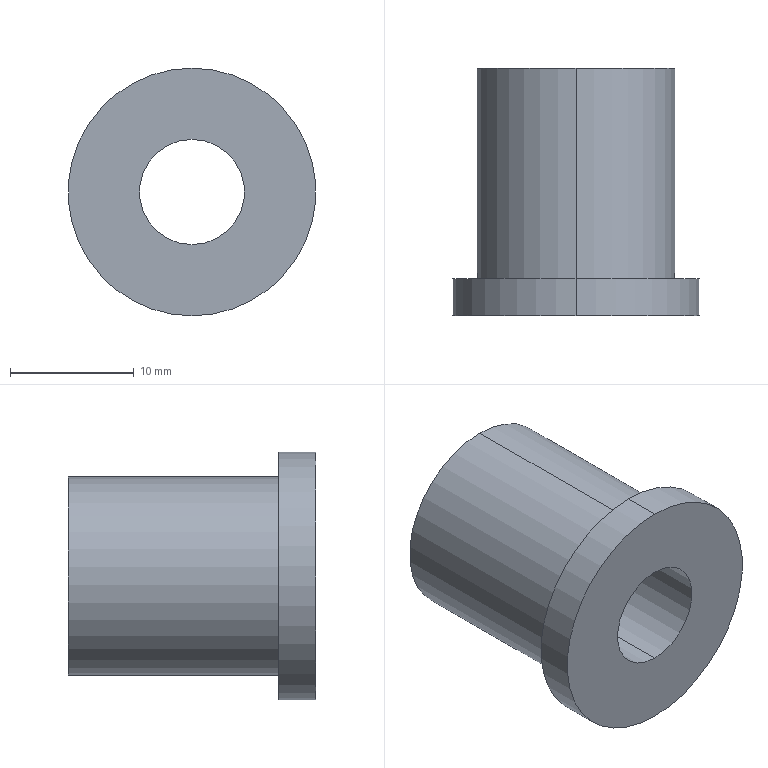Part | SolidWorks | features Extrusion 1, HoleWzd 1, ICE 1 | 1 solid | 9 faces | box 20 x 20 x 20 mm | volume 3226 mm3 | cylinder 6 | plane 3 | commonest cylinder face diameters 8.5 x2 16 x2 20 x2
STEP:
#1=CARTESIAN_POINT('',(0.,3.,-10.));
#2=VERTEX_POINT('',#1);
#3=CARTESIAN_POINT('',(0.,3.,10.));
#4=VERTEX_POINT('',#3);
#5=CARTESIAN_POINT('',(0.,3.,0.));
#6=DIRECTION('',(0.,-1.,0.));
#7=DIRECTION('',(0.,0.,-1.));
#8=AXIS2_PLACEMENT_3D('',#5,#6,#7);
#9=CIRCLE('',#8,10.);
#10=EDGE_CURVE('',#2,#4,#9,.T.);
#11=ORIENTED_EDGE('',*,*,#10,.T.);
#12=CARTESIAN_POINT('',(0.,0.,10.));
#13=VERTEX_POINT('',#12);
#14=CARTESIAN_POINT('',(0.,3.,10.));
#15=DIRECTION('',(0.,-1.,0.));
#16=VECTOR('',#15,1000.);
#17=LINE('',#14,#16);
#18=EDGE_CURVE('',#4,#13,#17,.T.);
#19=ORIENTED_EDGE('',*,*,#18,.T.);
#20=CARTESIAN_POINT('',(0.,0.,-10.));
#21=VERTEX_POINT('',#20);
#22=CARTESIAN_POINT('',(0.,0.,0.));
#23=DIRECTION('',(0.,-1.,0.));
#24=DIRECTION('',(0.,0.,-1.));
#25=AXIS2_PLACEMENT_3D('',#22,#23,#24);
#26=CIRCLE('',#25,10.);
#27=EDGE_CURVE('',#21,#13,#26,.T.);
#28=ORIENTED_EDGE('',*,*,#27,.F.);
#29=CARTESIAN_POINT('',(0.,3.,-10.));
#30=DIRECTION('',(0.,-1.,0.));
#31=VECTOR('',#30,1000.);
#32=LINE('',#29,#31);
#33=EDGE_CURVE('',#2,#21,#32,.T.);
#34=ORIENTED_EDGE('',*,*,#33,.F.);
#35=EDGE_LOOP('',(#11,#19,#28,#34));
#36=FACE_OUTER_BOUND('',#35,.T.);
#37=CARTESIAN_POINT('',(0.,3.,0.));
#38=DIRECTION('',(0.,-1.,0.));
#39=DIRECTION('',(0.,0.,-1.));
#40=AXIS2_PLACEMENT_3D('',#37,#38,#39);
#41=CYLINDRICAL_SURFACE('',#40,10.);
#42=ADVANCED_FACE('',(#36),#41,.T.);
#43=CARTESIAN_POINT('',(0.,0.,-4.25));
#44=VERTEX_POINT('',#43);
#45=CARTESIAN_POINT('',(0.,0.,4.25));
#46=VERTEX_POINT('',#45);
#47=CARTESIAN_POINT('',(0.,0.,0.));
#48=DIRECTION('',(0.,1.,0.));
#49=DIRECTION('',(0.,0.,1.));
#50=AXIS2_PLACEMENT_3D('',#47,#48,#49);
#51=CIRCLE('',#50,4.25);
#52=EDGE_CURVE('',#44,#46,#51,.T.);
#53=ORIENTED_EDGE('',*,*,#52,.F.);
#54=CARTESIAN_POINT('',(0.,20.,-4.25));
#55=VERTEX_POINT('',#54);
#56=CARTESIAN_POINT('',(0.,20.,-4.25));
#57=DIRECTION('',(0.,1.,0.));
#58=VECTOR('',#57,1000.);
#59=LINE('',#56,#58);
#60=EDGE_CURVE('',#44,#55,#59,.T.);
#61=ORIENTED_EDGE('',*,*,#60,.T.);
#62=CARTESIAN_POINT('',(0.,20.,4.25));
#63=VERTEX_POINT('',#62);
#64=CARTESIAN_POINT('',(0.,20.,0.));
#65=DIRECTION('',(0.,1.,0.));
#66=DIRECTION('',(0.,0.,1.));
#67=AXIS2_PLACEMENT_3D('',#64,#65,#66);
#68=CIRCLE('',#67,4.25);
#69=EDGE_CURVE('',#55,#63,#68,.T.);
#70=ORIENTED_EDGE('',*,*,#69,.T.);
#71=CARTESIAN_POINT('',(0.,20.,4.25));
#72=DIRECTION('',(0.,1.,0.));
#73=VECTOR('',#72,1000.);
#74=LINE('',#71,#73);
#75=EDGE_CURVE('',#46,#63,#74,.T.);
#76=ORIENTED_EDGE('',*,*,#75,.F.);
#77=EDGE_LOOP('',(#53,#61,#70,#76));
#78=FACE_OUTER_BOUND('',#77,.T.);
#79=CARTESIAN_POINT('',(0.,20.,0.));
#80=DIRECTION('',(0.,1.,0.));
#81=DIRECTION('',(0.,0.,1.));
#82=AXIS2_PLACEMENT_3D('',#79,#80,#81);
#83=CYLINDRICAL_SURFACE('',#82,4.25);
#84=ADVANCED_FACE('',(#78),#83,.F.);
#85=CARTESIAN_POINT('',(0.,20.,8.));
#86=VERTEX_POINT('',#85);
#87=CARTESIAN_POINT('',(0.,20.,-8.));
#88=VERTEX_POINT('',#87);
#89=CARTESIAN_POINT('',(0.,20.,0.));
#90=DIRECTION('',(0.,1.,0.));
#91=DIRECTION('',(0.,0.,1.));
#92=AXIS2_PLACEMENT_3D('',#89,#90,#91);
#93=CIRCLE('',#92,8.);
#94=EDGE_CURVE('',#86,#88,#93,.T.);
#95=ORIENTED_EDGE('',*,*,#94,.F.);
#96=CARTESIAN_POINT('',(0.,3.,8.));
#97=VERTEX_POINT('',#96);
#98=CARTESIAN_POINT('',(0.,20.,8.));
#99=DIRECTION('',(0.,-1.,0.));
#100=VECTOR('',#99,1000.);
#101=LINE('',#98,#100);
#102=EDGE_CURVE('',#86,#97,#101,.T.);
#103=ORIENTED_EDGE('',*,*,#102,.T.);
#104=CARTESIAN_POINT('',(0.,3.,-8.));
#105=VERTEX_POINT('',#104);
#106=CARTESIAN_POINT('',(0.,3.,0.));
#107=DIRECTION('',(0.,-1.,0.));
#108=DIRECTION('',(0.,0.,-1.));
#109=AXIS2_PLACEMENT_3D('',#106,#107,#108);
#110=CIRCLE('',#109,8.);
#111=EDGE_CURVE('',#105,#97,#110,.T.);
#112=ORIENTED_EDGE('',*,*,#111,.F.);
#113=CARTESIAN_POINT('',(0.,20.,-8.));
#114=DIRECTION('',(0.,-1.,0.));
#115=VECTOR('',#114,1000.);
#116=LINE('',#113,#115);
#117=EDGE_CURVE('',#88,#105,#116,.T.);
#118=ORIENTED_EDGE('',*,*,#117,.F.);
#119=EDGE_LOOP('',(#95,#103,#112,#118));
#120=FACE_OUTER_BOUND('',#119,.T.);
#121=CARTESIAN_POINT('',(0.,20.,0.));
#122=DIRECTION('',(0.,-1.,0.));
#123=DIRECTION('',(0.,0.,-1.));
#124=AXIS2_PLACEMENT_3D('',#121,#122,#123);
#125=CYLINDRICAL_SURFACE('',#124,8.);
#126=ADVANCED_FACE('',(#120),#125,.T.);
#127=ORIENTED_EDGE('',*,*,#102,.F.);
#128=CARTESIAN_POINT('',(0.,20.,0.));
#129=DIRECTION('',(0.,1.,0.));
#130=DIRECTION('',(0.,0.,1.));
#131=AXIS2_PLACEMENT_3D('',#128,#129,#130);
#132=CIRCLE('',#131,8.);
#133=EDGE_CURVE('',#88,#86,#132,.T.);
#134=ORIENTED_EDGE('',*,*,#133,.F.);
#135=ORIENTED_EDGE('',*,*,#117,.T.);
#136=CARTESIAN_POINT('',(0.,3.,0.));
#137=DIRECTION('',(0.,-1.,0.));
#138=DIRECTION('',(0.,0.,-1.));
#139=AXIS2_PLACEMENT_3D('',#136,#137,#138);
#140=CIRCLE('',#139,8.);
#141=EDGE_CURVE('',#97,#105,#140,.T.);
#142=ORIENTED_EDGE('',*,*,#141,.F.);
#143=EDGE_LOOP('',(#127,#134,#135,#142));
#144=FACE_OUTER_BOUND('',#143,.T.);
#145=CARTESIAN_POINT('',(0.,20.,0.));
#146=DIRECTION('',(0.,-1.,0.));
#147=DIRECTION('',(0.,0.,-1.));
#148=AXIS2_PLACEMENT_3D('',#145,#146,#147);
#149=CYLINDRICAL_SURFACE('',#148,8.);
#150=ADVANCED_FACE('',(#144),#149,.T.);
#151=CARTESIAN_POINT('',(0.,20.,0.));
#152=DIRECTION('',(0.,1.,0.));
#153=DIRECTION('',(0.,0.,1.));
#154=AXIS2_PLACEMENT_3D('',#151,#152,#153);
#155=CIRCLE('',#154,4.25);
#156=EDGE_CURVE('',#63,#55,#155,.T.);
#157=ORIENTED_EDGE('',*,*,#156,.F.);
#158=ORIENTED_EDGE('',*,*,#69,.F.);
#159=EDGE_LOOP('',(#157,#158));
#160=FACE_BOUND('',#159,.T.);
#161=ORIENTED_EDGE('',*,*,#133,.T.);
#162=ORIENTED_EDGE('',*,*,#94,.T.);
#163=EDGE_LOOP('',(#161,#162));
#164=FACE_OUTER_BOUND('',#163,.T.);
#165=CARTESIAN_POINT('',(0.,20.,0.));
#166=DIRECTION('',(0.,1.,0.));
#167=DIRECTION('',(0.,0.,1.));
#168=AXIS2_PLACEMENT_3D('',#165,#166,#167);
#169=PLANE('',#168);
#170=ADVANCED_FACE('',(#160,#164),#169,.T.);
#171=CARTESIAN_POINT('',(0.,0.,0.));
#172=DIRECTION('',(0.,1.,0.));
#173=DIRECTION('',(0.,0.,1.));
#174=AXIS2_PLACEMENT_3D('',#171,#172,#173);
#175=CIRCLE('',#174,4.25);
#176=EDGE_CURVE('',#46,#44,#175,.T.);
#177=ORIENTED_EDGE('',*,*,#176,.T.);
#178=ORIENTED_EDGE('',*,*,#52,.T.);
#179=EDGE_LOOP('',(#177,#178));
#180=FACE_BOUND('',#179,.T.);
#181=ORIENTED_EDGE('',*,*,#27,.T.);
#182=CARTESIAN_POINT('',(0.,0.,0.));
#183=DIRECTION('',(0.,-1.,0.));
#184=DIRECTION('',(0.,0.,-1.));
#185=AXIS2_PLACEMENT_3D('',#182,#183,#184);
#186=CIRCLE('',#185,10.);
#187=EDGE_CURVE('',#13,#21,#186,.T.);
#188=ORIENTED_EDGE('',*,*,#187,.T.);
#189=EDGE_LOOP('',(#181,#188));
#190=FACE_OUTER_BOUND('',#189,.T.);
#191=CARTESIAN_POINT('',(0.,0.,0.));
#192=DIRECTION('',(0.,1.,0.));
#193=DIRECTION('',(0.,0.,1.));
#194=AXIS2_PLACEMENT_3D('',#191,#192,#193);
#195=PLANE('',#194);
#196=ADVANCED_FACE('',(#180,#190),#195,.F.);
#197=ORIENTED_EDGE('',*,*,#60,.F.);
#198=ORIENTED_EDGE('',*,*,#176,.F.);
#199=ORIENTED_EDGE('',*,*,#75,.T.);
#200=ORIENTED_EDGE('',*,*,#156,.T.);
#201=EDGE_LOOP('',(#197,#198,#199,#200));
#202=FACE_OUTER_BOUND('',#201,.T.);
#203=CARTESIAN_POINT('',(0.,20.,0.));
#204=DIRECTION('',(0.,1.,0.));
#205=DIRECTION('',(0.,0.,1.));
#206=AXIS2_PLACEMENT_3D('',#203,#204,#205);
#207=CYLINDRICAL_SURFACE('',#206,4.25);
#208=ADVANCED_FACE('',(#202),#207,.F.);
#209=ORIENTED_EDGE('',*,*,#18,.F.);
#210=CARTESIAN_POINT('',(0.,3.,0.));
#211=DIRECTION('',(0.,-1.,0.));
#212=DIRECTION('',(0.,0.,-1.));
#213=AXIS2_PLACEMENT_3D('',#210,#211,#212);
#214=CIRCLE('',#213,10.);
#215=EDGE_CURVE('',#4,#2,#214,.T.);
#216=ORIENTED_EDGE('',*,*,#215,.T.);
#217=ORIENTED_EDGE('',*,*,#33,.T.);
#218=ORIENTED_EDGE('',*,*,#187,.F.);
#219=EDGE_LOOP('',(#209,#216,#217,#218));
#220=FACE_OUTER_BOUND('',#219,.T.);
#221=CARTESIAN_POINT('',(0.,3.,0.));
#222=DIRECTION('',(0.,-1.,0.));
#223=DIRECTION('',(0.,0.,-1.));
#224=AXIS2_PLACEMENT_3D('',#221,#222,#223);
#225=CYLINDRICAL_SURFACE('',#224,10.);
#226=ADVANCED_FACE('',(#220),#225,.T.);
#227=ORIENTED_EDGE('',*,*,#111,.T.);
#228=ORIENTED_EDGE('',*,*,#141,.T.);
#229=EDGE_LOOP('',(#227,#228));
#230=FACE_BOUND('',#229,.T.);
#231=ORIENTED_EDGE('',*,*,#10,.F.);
#232=ORIENTED_EDGE('',*,*,#215,.F.);
#233=EDGE_LOOP('',(#231,#232));
#234=FACE_OUTER_BOUND('',#233,.T.);
#235=CARTESIAN_POINT('',(0.,3.,0.));
#236=DIRECTION('',(0.,-1.,0.));
#237=DIRECTION('',(0.,0.,-1.));
#238=AXIS2_PLACEMENT_3D('',#235,#236,#237);
#239=PLANE('',#238);
#240=ADVANCED_FACE('',(#230,#234),#239,.F.);
#241=CLOSED_SHELL('',(#42,#84,#126,#150,#170,#196,#208,#226,#240));
#242=MANIFOLD_SOLID_BREP('',#241);
#243=CARTESIAN_POINT('',(0.,0.,0.));
#244=DIRECTION('',(0.,0.,1.));
#245=DIRECTION('',(1.,0.,0.));
#246=AXIS2_PLACEMENT_3D('',#243,#244,#245);
#247=(LENGTH_UNIT()NAMED_UNIT(*)SI_UNIT(.MILLI.,.METRE.));
#248=UNCERTAINTY_MEASURE_WITH_UNIT(LENGTH_MEASURE(0.00001),#247,'','');
#249=(NAMED_UNIT(*)PLANE_ANGLE_UNIT()SI_UNIT($,.RADIAN.));
#250=(NAMED_UNIT(*)SI_UNIT($,.STERADIAN.)SOLID_ANGLE_UNIT());
#251=(GEOMETRIC_REPRESENTATION_CONTEXT(3)GLOBAL_UNCERTAINTY_ASSIGNED_CONTEXT((#248))GLOBAL_UNIT_ASSIGNED_CONTEXT((#247,#249,#250))REPRESENTATION_CONTEXT('',''));
#252=ADVANCED_BREP_SHAPE_REPRESENTATION('',(#242,#246),#251);